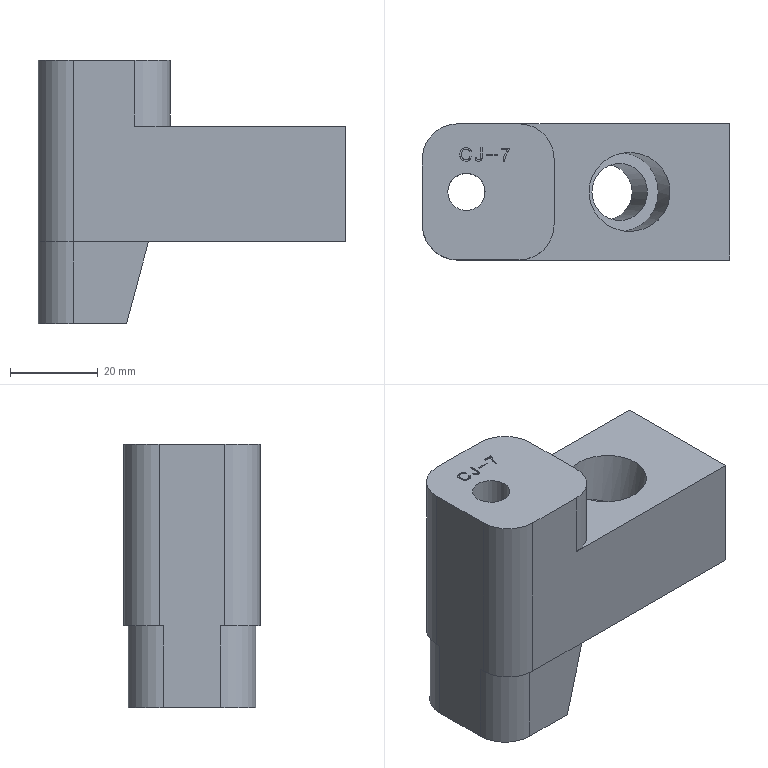Part | STEP file | solid 6 | 1 solid | 49 faces | box 70 x 31 x 60 mm | volume 72182 mm3 | plane 33 | cylinder 10 | other 6 | commonest cylinder face diameters 16 x6 8.5 x1 13 x1 14 x1 18 x1